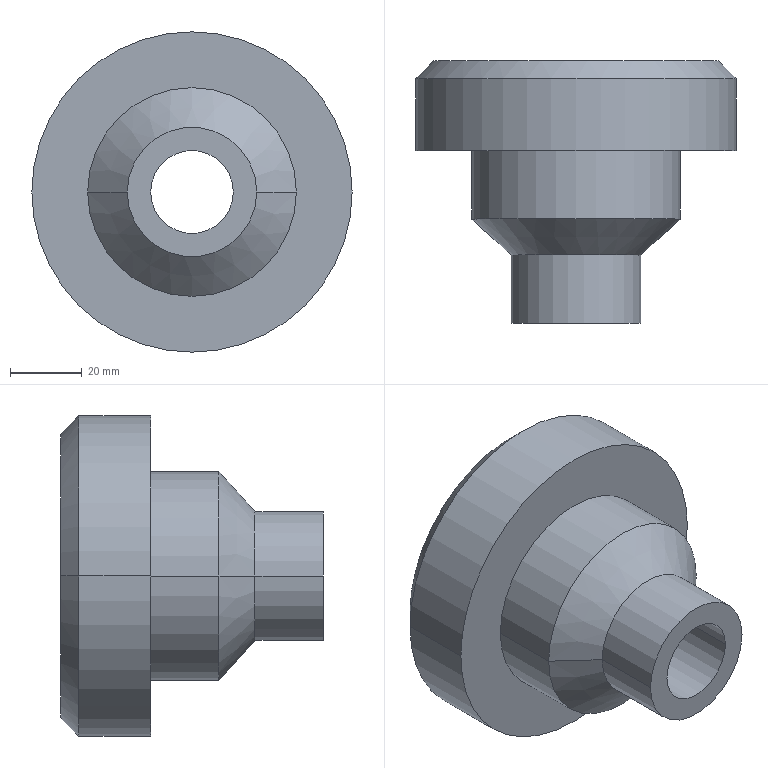Part | SolidWorks | features Chamfer 1, Revolution 1 | 1 solid | 15 faces | box 89 x 73 x 89 mm | volume 209040 mm3 | cylinder 8 | cone 4 | plane 3 | commonest cylinder face diameters 23 x2 36 x2 58 x2 89 x2
STEP:
#1=CARTESIAN_POINT('',(-39.5,73.,0.));
#2=VERTEX_POINT('',#1);
#3=CARTESIAN_POINT('',(39.5,73.,0.));
#4=VERTEX_POINT('',#3);
#5=CARTESIAN_POINT('',(0.,73.,0.));
#6=DIRECTION('',(0.,1.,0.));
#7=DIRECTION('',(-1.,0.,0.));
#8=AXIS2_PLACEMENT_3D('',#5,#6,#7);
#9=CIRCLE('',#8,39.5);
#10=EDGE_CURVE('',#2,#4,#9,.T.);
#11=ORIENTED_EDGE('',*,*,#10,.F.);
#12=CARTESIAN_POINT('',(-44.5,68.,0.));
#13=VERTEX_POINT('',#12);
#14=CARTESIAN_POINT('',(-44.5,68.,0.));
#15=DIRECTION('',(-0.7071,-0.7071,0.));
#16=VECTOR('',#15,1000.);
#17=LINE('',#14,#16);
#18=EDGE_CURVE('',#2,#13,#17,.T.);
#19=ORIENTED_EDGE('',*,*,#18,.T.);
#20=CARTESIAN_POINT('',(44.5,68.,0.));
#21=VERTEX_POINT('',#20);
#22=CARTESIAN_POINT('',(0.,68.,0.));
#23=DIRECTION('',(0.,-1.,0.));
#24=DIRECTION('',(-1.,0.,0.));
#25=AXIS2_PLACEMENT_3D('',#22,#23,#24);
#26=CIRCLE('',#25,44.5);
#27=EDGE_CURVE('',#21,#13,#26,.T.);
#28=ORIENTED_EDGE('',*,*,#27,.F.);
#29=CARTESIAN_POINT('',(44.5,68.,0.));
#30=DIRECTION('',(0.7071,-0.7071,0.));
#31=VECTOR('',#30,1000.);
#32=LINE('',#29,#31);
#33=EDGE_CURVE('',#4,#21,#32,.T.);
#34=ORIENTED_EDGE('',*,*,#33,.F.);
#35=EDGE_LOOP('',(#11,#19,#28,#34));
#36=FACE_OUTER_BOUND('',#35,.T.);
#37=CARTESIAN_POINT('',(0.,68.,0.));
#38=DIRECTION('',(0.,-1.,0.));
#39=DIRECTION('',(1.,0.,0.));
#40=AXIS2_PLACEMENT_3D('',#37,#38,#39);
#41=CONICAL_SURFACE('',#40,44.5,0.7854);
#42=ADVANCED_FACE('',(#36),#41,.T.);
#43=CARTESIAN_POINT('',(18.,19.,0.));
#44=VERTEX_POINT('',#43);
#45=CARTESIAN_POINT('',(-18.,19.,0.));
#46=VERTEX_POINT('',#45);
#47=CARTESIAN_POINT('',(0.,19.,0.));
#48=DIRECTION('',(0.,-1.,0.));
#49=DIRECTION('',(1.,0.,0.));
#50=AXIS2_PLACEMENT_3D('',#47,#48,#49);
#51=CIRCLE('',#50,18.);
#52=EDGE_CURVE('',#44,#46,#51,.T.);
#53=ORIENTED_EDGE('',*,*,#52,.T.);
#54=CARTESIAN_POINT('',(-18.,0.,0.));
#55=VERTEX_POINT('',#54);
#56=CARTESIAN_POINT('',(-18.,-693.799,0.));
#57=DIRECTION('',(0.,-1.,0.));
#58=VECTOR('',#57,1000.);
#59=LINE('',#56,#58);
#60=EDGE_CURVE('',#46,#55,#59,.T.);
#61=ORIENTED_EDGE('',*,*,#60,.T.);
#62=CARTESIAN_POINT('',(18.,0.,0.));
#63=VERTEX_POINT('',#62);
#64=CARTESIAN_POINT('',(0.,0.,0.));
#65=DIRECTION('',(0.,-1.,0.));
#66=DIRECTION('',(1.,0.,0.));
#67=AXIS2_PLACEMENT_3D('',#64,#65,#66);
#68=CIRCLE('',#67,18.);
#69=EDGE_CURVE('',#63,#55,#68,.T.);
#70=ORIENTED_EDGE('',*,*,#69,.F.);
#71=CARTESIAN_POINT('',(18.,-693.799,0.));
#72=DIRECTION('',(0.,-1.,0.));
#73=VECTOR('',#72,1000.);
#74=LINE('',#71,#73);
#75=EDGE_CURVE('',#44,#63,#74,.T.);
#76=ORIENTED_EDGE('',*,*,#75,.F.);
#77=EDGE_LOOP('',(#53,#61,#70,#76));
#78=FACE_OUTER_BOUND('',#77,.T.);
#79=CARTESIAN_POINT('',(0.,-693.799,0.));
#80=DIRECTION('',(0.,-1.,0.));
#81=DIRECTION('',(1.,0.,0.));
#82=AXIS2_PLACEMENT_3D('',#79,#80,#81);
#83=CYLINDRICAL_SURFACE('',#82,18.);
#84=ADVANCED_FACE('',(#78),#83,.T.);
#85=ORIENTED_EDGE('',*,*,#52,.F.);
#86=CARTESIAN_POINT('',(29.,29.,0.));
#87=VERTEX_POINT('',#86);
#88=CARTESIAN_POINT('',(18.,19.,0.));
#89=DIRECTION('',(0.7399,0.6727,0.));
#90=VECTOR('',#89,1000.);
#91=LINE('',#88,#90);
#92=EDGE_CURVE('',#44,#87,#91,.T.);
#93=ORIENTED_EDGE('',*,*,#92,.T.);
#94=CARTESIAN_POINT('',(-29.,29.,0.));
#95=VERTEX_POINT('',#94);
#96=CARTESIAN_POINT('',(0.,29.,0.));
#97=DIRECTION('',(0.,-1.,0.));
#98=DIRECTION('',(1.,0.,0.));
#99=AXIS2_PLACEMENT_3D('',#96,#97,#98);
#100=CIRCLE('',#99,29.);
#101=EDGE_CURVE('',#87,#95,#100,.T.);
#102=ORIENTED_EDGE('',*,*,#101,.T.);
#103=CARTESIAN_POINT('',(-18.,19.,0.));
#104=DIRECTION('',(-0.7399,0.6727,0.));
#105=VECTOR('',#104,1000.);
#106=LINE('',#103,#105);
#107=EDGE_CURVE('',#46,#95,#106,.T.);
#108=ORIENTED_EDGE('',*,*,#107,.F.);
#109=EDGE_LOOP('',(#85,#93,#102,#108));
#110=FACE_OUTER_BOUND('',#109,.T.);
#111=CARTESIAN_POINT('',(0.,19.,0.));
#112=DIRECTION('',(0.,1.,0.));
#113=DIRECTION('',(-1.,0.,0.));
#114=AXIS2_PLACEMENT_3D('',#111,#112,#113);
#115=CONICAL_SURFACE('',#114,18.,0.833);
#116=ADVANCED_FACE('',(#110),#115,.T.);
#117=CARTESIAN_POINT('',(29.,48.,0.));
#118=VERTEX_POINT('',#117);
#119=CARTESIAN_POINT('',(-29.,48.,0.));
#120=VERTEX_POINT('',#119);
#121=CARTESIAN_POINT('',(0.,48.,0.));
#122=DIRECTION('',(0.,-1.,0.));
#123=DIRECTION('',(1.,0.,0.));
#124=AXIS2_PLACEMENT_3D('',#121,#122,#123);
#125=CIRCLE('',#124,29.);
#126=EDGE_CURVE('',#118,#120,#125,.T.);
#127=ORIENTED_EDGE('',*,*,#126,.T.);
#128=CARTESIAN_POINT('',(-29.,-693.799,0.));
#129=DIRECTION('',(0.,-1.,0.));
#130=VECTOR('',#129,1000.);
#131=LINE('',#128,#130);
#132=EDGE_CURVE('',#120,#95,#131,.T.);
#133=ORIENTED_EDGE('',*,*,#132,.T.);
#134=ORIENTED_EDGE('',*,*,#101,.F.);
#135=CARTESIAN_POINT('',(29.,-693.799,0.));
#136=DIRECTION('',(0.,-1.,0.));
#137=VECTOR('',#136,1000.);
#138=LINE('',#135,#137);
#139=EDGE_CURVE('',#118,#87,#138,.T.);
#140=ORIENTED_EDGE('',*,*,#139,.F.);
#141=EDGE_LOOP('',(#127,#133,#134,#140));
#142=FACE_OUTER_BOUND('',#141,.T.);
#143=CARTESIAN_POINT('',(0.,-693.799,0.));
#144=DIRECTION('',(0.,-1.,0.));
#145=DIRECTION('',(1.,0.,0.));
#146=AXIS2_PLACEMENT_3D('',#143,#144,#145);
#147=CYLINDRICAL_SURFACE('',#146,29.);
#148=ADVANCED_FACE('',(#142),#147,.T.);
#149=ORIENTED_EDGE('',*,*,#27,.T.);
#150=CARTESIAN_POINT('',(-44.5,48.,0.));
#151=VERTEX_POINT('',#150);
#152=CARTESIAN_POINT('',(-44.5,-693.799,0.));
#153=DIRECTION('',(0.,-1.,0.));
#154=VECTOR('',#153,1000.);
#155=LINE('',#152,#154);
#156=EDGE_CURVE('',#13,#151,#155,.T.);
#157=ORIENTED_EDGE('',*,*,#156,.T.);
#158=CARTESIAN_POINT('',(44.5,48.,0.));
#159=VERTEX_POINT('',#158);
#160=CARTESIAN_POINT('',(0.,48.,0.));
#161=DIRECTION('',(0.,-1.,0.));
#162=DIRECTION('',(1.,0.,0.));
#163=AXIS2_PLACEMENT_3D('',#160,#161,#162);
#164=CIRCLE('',#163,44.5);
#165=EDGE_CURVE('',#159,#151,#164,.T.);
#166=ORIENTED_EDGE('',*,*,#165,.F.);
#167=CARTESIAN_POINT('',(44.5,-693.799,0.));
#168=DIRECTION('',(0.,-1.,0.));
#169=VECTOR('',#168,1000.);
#170=LINE('',#167,#169);
#171=EDGE_CURVE('',#21,#159,#170,.T.);
#172=ORIENTED_EDGE('',*,*,#171,.F.);
#173=EDGE_LOOP('',(#149,#157,#166,#172));
#174=FACE_OUTER_BOUND('',#173,.T.);
#175=CARTESIAN_POINT('',(0.,-693.799,0.));
#176=DIRECTION('',(0.,-1.,0.));
#177=DIRECTION('',(1.,0.,0.));
#178=AXIS2_PLACEMENT_3D('',#175,#176,#177);
#179=CYLINDRICAL_SURFACE('',#178,44.5);
#180=ADVANCED_FACE('',(#174),#179,.T.);
#181=CARTESIAN_POINT('',(-11.5,73.,0.));
#182=VERTEX_POINT('',#181);
#183=CARTESIAN_POINT('',(11.5,73.,0.));
#184=VERTEX_POINT('',#183);
#185=CARTESIAN_POINT('',(0.,73.,0.));
#186=DIRECTION('',(0.,-1.,0.));
#187=DIRECTION('',(1.,0.,0.));
#188=AXIS2_PLACEMENT_3D('',#185,#186,#187);
#189=CIRCLE('',#188,11.5);
#190=EDGE_CURVE('',#182,#184,#189,.T.);
#191=ORIENTED_EDGE('',*,*,#190,.F.);
#192=CARTESIAN_POINT('',(-11.5,0.,0.));
#193=VERTEX_POINT('',#192);
#194=CARTESIAN_POINT('',(-11.5,-693.799,0.));
#195=DIRECTION('',(0.,-1.,0.));
#196=VECTOR('',#195,1000.);
#197=LINE('',#194,#196);
#198=EDGE_CURVE('',#182,#193,#197,.T.);
#199=ORIENTED_EDGE('',*,*,#198,.T.);
#200=CARTESIAN_POINT('',(11.5,0.,0.));
#201=VERTEX_POINT('',#200);
#202=CARTESIAN_POINT('',(0.,0.,0.));
#203=DIRECTION('',(0.,-1.,0.));
#204=DIRECTION('',(1.,0.,0.));
#205=AXIS2_PLACEMENT_3D('',#202,#203,#204);
#206=CIRCLE('',#205,11.5);
#207=EDGE_CURVE('',#193,#201,#206,.T.);
#208=ORIENTED_EDGE('',*,*,#207,.T.);
#209=CARTESIAN_POINT('',(11.5,-693.799,0.));
#210=DIRECTION('',(0.,-1.,0.));
#211=VECTOR('',#210,1000.);
#212=LINE('',#209,#211);
#213=EDGE_CURVE('',#184,#201,#212,.T.);
#214=ORIENTED_EDGE('',*,*,#213,.F.);
#215=EDGE_LOOP('',(#191,#199,#208,#214));
#216=FACE_OUTER_BOUND('',#215,.T.);
#217=CARTESIAN_POINT('',(0.,-693.799,0.));
#218=DIRECTION('',(0.,-1.,0.));
#219=DIRECTION('',(1.,0.,0.));
#220=AXIS2_PLACEMENT_3D('',#217,#218,#219);
#221=CYLINDRICAL_SURFACE('',#220,11.5);
#222=ADVANCED_FACE('',(#216),#221,.F.);
#223=ORIENTED_EDGE('',*,*,#69,.T.);
#224=CARTESIAN_POINT('',(0.,0.,0.));
#225=DIRECTION('',(0.,-1.,0.));
#226=DIRECTION('',(1.,0.,0.));
#227=AXIS2_PLACEMENT_3D('',#224,#225,#226);
#228=CIRCLE('',#227,18.);
#229=EDGE_CURVE('',#55,#63,#228,.T.);
#230=ORIENTED_EDGE('',*,*,#229,.T.);
#231=EDGE_LOOP('',(#223,#230));
#232=FACE_OUTER_BOUND('',#231,.T.);
#233=CARTESIAN_POINT('',(0.,0.,0.));
#234=DIRECTION('',(0.,-1.,0.));
#235=DIRECTION('',(1.,0.,0.));
#236=AXIS2_PLACEMENT_3D('',#233,#234,#235);
#237=CIRCLE('',#236,11.5);
#238=EDGE_CURVE('',#201,#193,#237,.T.);
#239=ORIENTED_EDGE('',*,*,#238,.F.);
#240=ORIENTED_EDGE('',*,*,#207,.F.);
#241=EDGE_LOOP('',(#239,#240));
#242=FACE_BOUND('',#241,.T.);
#243=CARTESIAN_POINT('',(18.,0.,0.));
#244=DIRECTION('',(0.,-1.,0.));
#245=DIRECTION('',(1.,0.,0.));
#246=AXIS2_PLACEMENT_3D('',#243,#244,#245);
#247=PLANE('',#246);
#248=ADVANCED_FACE('',(#232,#242),#247,.T.);
#249=ORIENTED_EDGE('',*,*,#198,.F.);
#250=CARTESIAN_POINT('',(0.,73.,0.));
#251=DIRECTION('',(0.,-1.,0.));
#252=DIRECTION('',(1.,0.,0.));
#253=AXIS2_PLACEMENT_3D('',#250,#251,#252);
#254=CIRCLE('',#253,11.5);
#255=EDGE_CURVE('',#184,#182,#254,.T.);
#256=ORIENTED_EDGE('',*,*,#255,.F.);
#257=ORIENTED_EDGE('',*,*,#213,.T.);
#258=ORIENTED_EDGE('',*,*,#238,.T.);
#259=EDGE_LOOP('',(#249,#256,#257,#258));
#260=FACE_OUTER_BOUND('',#259,.T.);
#261=CARTESIAN_POINT('',(0.,-693.799,0.));
#262=DIRECTION('',(0.,-1.,0.));
#263=DIRECTION('',(1.,0.,0.));
#264=AXIS2_PLACEMENT_3D('',#261,#262,#263);
#265=CYLINDRICAL_SURFACE('',#264,11.5);
#266=ADVANCED_FACE('',(#260),#265,.F.);
#267=CARTESIAN_POINT('',(0.,73.,0.));
#268=DIRECTION('',(0.,1.,0.));
#269=DIRECTION('',(-1.,0.,0.));
#270=AXIS2_PLACEMENT_3D('',#267,#268,#269);
#271=CIRCLE('',#270,39.5);
#272=EDGE_CURVE('',#4,#2,#271,.T.);
#273=ORIENTED_EDGE('',*,*,#272,.T.);
#274=ORIENTED_EDGE('',*,*,#10,.T.);
#275=EDGE_LOOP('',(#273,#274));
#276=FACE_OUTER_BOUND('',#275,.T.);
#277=ORIENTED_EDGE('',*,*,#255,.T.);
#278=ORIENTED_EDGE('',*,*,#190,.T.);
#279=EDGE_LOOP('',(#277,#278));
#280=FACE_BOUND('',#279,.T.);
#281=CARTESIAN_POINT('',(11.5,73.,0.));
#282=DIRECTION('',(0.,1.,0.));
#283=DIRECTION('',(-1.,0.,0.));
#284=AXIS2_PLACEMENT_3D('',#281,#282,#283);
#285=PLANE('',#284);
#286=ADVANCED_FACE('',(#276,#280),#285,.T.);
#287=ORIENTED_EDGE('',*,*,#156,.F.);
#288=CARTESIAN_POINT('',(0.,68.,0.));
#289=DIRECTION('',(0.,-1.,0.));
#290=DIRECTION('',(-1.,0.,0.));
#291=AXIS2_PLACEMENT_3D('',#288,#289,#290);
#292=CIRCLE('',#291,44.5);
#293=EDGE_CURVE('',#13,#21,#292,.T.);
#294=ORIENTED_EDGE('',*,*,#293,.T.);
#295=ORIENTED_EDGE('',*,*,#171,.T.);
#296=CARTESIAN_POINT('',(0.,48.,0.));
#297=DIRECTION('',(0.,-1.,0.));
#298=DIRECTION('',(1.,0.,0.));
#299=AXIS2_PLACEMENT_3D('',#296,#297,#298);
#300=CIRCLE('',#299,44.5);
#301=EDGE_CURVE('',#151,#159,#300,.T.);
#302=ORIENTED_EDGE('',*,*,#301,.F.);
#303=EDGE_LOOP('',(#287,#294,#295,#302));
#304=FACE_OUTER_BOUND('',#303,.T.);
#305=CARTESIAN_POINT('',(0.,-693.799,0.));
#306=DIRECTION('',(0.,-1.,0.));
#307=DIRECTION('',(1.,0.,0.));
#308=AXIS2_PLACEMENT_3D('',#305,#306,#307);
#309=CYLINDRICAL_SURFACE('',#308,44.5);
#310=ADVANCED_FACE('',(#304),#309,.T.);
#311=ORIENTED_EDGE('',*,*,#165,.T.);
#312=ORIENTED_EDGE('',*,*,#301,.T.);
#313=EDGE_LOOP('',(#311,#312));
#314=FACE_OUTER_BOUND('',#313,.T.);
#315=ORIENTED_EDGE('',*,*,#126,.F.);
#316=CARTESIAN_POINT('',(0.,48.,0.));
#317=DIRECTION('',(0.,-1.,0.));
#318=DIRECTION('',(1.,0.,0.));
#319=AXIS2_PLACEMENT_3D('',#316,#317,#318);
#320=CIRCLE('',#319,29.);
#321=EDGE_CURVE('',#120,#118,#320,.T.);
#322=ORIENTED_EDGE('',*,*,#321,.F.);
#323=EDGE_LOOP('',(#315,#322));
#324=FACE_BOUND('',#323,.T.);
#325=CARTESIAN_POINT('',(44.5,48.,0.));
#326=DIRECTION('',(0.,-1.,0.));
#327=DIRECTION('',(1.,0.,0.));
#328=AXIS2_PLACEMENT_3D('',#325,#326,#327);
#329=PLANE('',#328);
#330=ADVANCED_FACE('',(#314,#324),#329,.T.);
#331=ORIENTED_EDGE('',*,*,#132,.F.);
#332=ORIENTED_EDGE('',*,*,#321,.T.);
#333=ORIENTED_EDGE('',*,*,#139,.T.);
#334=CARTESIAN_POINT('',(0.,29.,0.));
#335=DIRECTION('',(0.,-1.,0.));
#336=DIRECTION('',(1.,0.,0.));
#337=AXIS2_PLACEMENT_3D('',#334,#335,#336);
#338=CIRCLE('',#337,29.);
#339=EDGE_CURVE('',#95,#87,#338,.T.);
#340=ORIENTED_EDGE('',*,*,#339,.F.);
#341=EDGE_LOOP('',(#331,#332,#333,#340));
#342=FACE_OUTER_BOUND('',#341,.T.);
#343=CARTESIAN_POINT('',(0.,-693.799,0.));
#344=DIRECTION('',(0.,-1.,0.));
#345=DIRECTION('',(1.,0.,0.));
#346=AXIS2_PLACEMENT_3D('',#343,#344,#345);
#347=CYLINDRICAL_SURFACE('',#346,29.);
#348=ADVANCED_FACE('',(#342),#347,.T.);
#349=ORIENTED_EDGE('',*,*,#92,.F.);
#350=CARTESIAN_POINT('',(0.,19.,0.));
#351=DIRECTION('',(0.,-1.,0.));
#352=DIRECTION('',(1.,0.,0.));
#353=AXIS2_PLACEMENT_3D('',#350,#351,#352);
#354=CIRCLE('',#353,18.);
#355=EDGE_CURVE('',#46,#44,#354,.T.);
#356=ORIENTED_EDGE('',*,*,#355,.F.);
#357=ORIENTED_EDGE('',*,*,#107,.T.);
#358=ORIENTED_EDGE('',*,*,#339,.T.);
#359=EDGE_LOOP('',(#349,#356,#357,#358));
#360=FACE_OUTER_BOUND('',#359,.T.);
#361=CARTESIAN_POINT('',(0.,19.,0.));
#362=DIRECTION('',(0.,1.,0.));
#363=DIRECTION('',(-1.,0.,0.));
#364=AXIS2_PLACEMENT_3D('',#361,#362,#363);
#365=CONICAL_SURFACE('',#364,18.,0.833);
#366=ADVANCED_FACE('',(#360),#365,.T.);
#367=ORIENTED_EDGE('',*,*,#60,.F.);
#368=ORIENTED_EDGE('',*,*,#355,.T.);
#369=ORIENTED_EDGE('',*,*,#75,.T.);
#370=ORIENTED_EDGE('',*,*,#229,.F.);
#371=EDGE_LOOP('',(#367,#368,#369,#370));
#372=FACE_OUTER_BOUND('',#371,.T.);
#373=CARTESIAN_POINT('',(0.,-693.799,0.));
#374=DIRECTION('',(0.,-1.,0.));
#375=DIRECTION('',(1.,0.,0.));
#376=AXIS2_PLACEMENT_3D('',#373,#374,#375);
#377=CYLINDRICAL_SURFACE('',#376,18.);
#378=ADVANCED_FACE('',(#372),#377,.T.);
#379=ORIENTED_EDGE('',*,*,#18,.F.);
#380=ORIENTED_EDGE('',*,*,#272,.F.);
#381=ORIENTED_EDGE('',*,*,#33,.T.);
#382=ORIENTED_EDGE('',*,*,#293,.F.);
#383=EDGE_LOOP('',(#379,#380,#381,#382));
#384=FACE_OUTER_BOUND('',#383,.T.);
#385=CARTESIAN_POINT('',(0.,68.,0.));
#386=DIRECTION('',(0.,-1.,0.));
#387=DIRECTION('',(1.,0.,0.));
#388=AXIS2_PLACEMENT_3D('',#385,#386,#387);
#389=CONICAL_SURFACE('',#388,44.5,0.7854);
#390=ADVANCED_FACE('',(#384),#389,.T.);
#391=CLOSED_SHELL('',(#42,#84,#116,#148,#180,#222,#248,#266,#286,#310,#330,#348,#366,#378,#390));
#392=MANIFOLD_SOLID_BREP('',#391);
#393=CARTESIAN_POINT('',(0.,0.,0.));
#394=DIRECTION('',(0.,0.,1.));
#395=DIRECTION('',(1.,0.,0.));
#396=AXIS2_PLACEMENT_3D('',#393,#394,#395);
#397=(LENGTH_UNIT()NAMED_UNIT(*)SI_UNIT(.MILLI.,.METRE.));
#398=UNCERTAINTY_MEASURE_WITH_UNIT(LENGTH_MEASURE(0.00001),#397,'','');
#399=(NAMED_UNIT(*)PLANE_ANGLE_UNIT()SI_UNIT($,.RADIAN.));
#400=(NAMED_UNIT(*)SI_UNIT($,.STERADIAN.)SOLID_ANGLE_UNIT());
#401=(GEOMETRIC_REPRESENTATION_CONTEXT(3)GLOBAL_UNCERTAINTY_ASSIGNED_CONTEXT((#398))GLOBAL_UNIT_ASSIGNED_CONTEXT((#397,#399,#400))REPRESENTATION_CONTEXT('',''));
#402=ADVANCED_BREP_SHAPE_REPRESENTATION('',(#392,#396),#401);